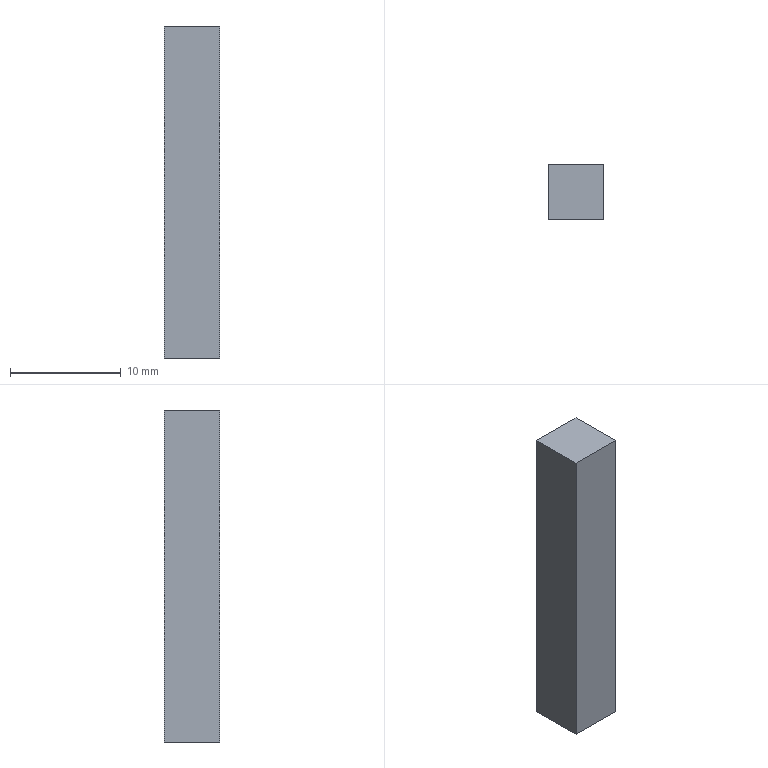Part | STEP file | BCC3 H16_16 | 1 solid | 6 faces | box 5 x 5 x 30 mm | volume 750 mm3 | plane 6
STEP:
#1=CARTESIAN_POINT('',(0.,0.,0.));
#2=DIRECTION('',(0.,0.,1.));
#3=DIRECTION('',(1.,0.,0.));
#4=AXIS2_PLACEMENT_3D('',#1,#2,#3);
#5=CARTESIAN_POINT('',(-2.5,2.5,-15.));
#6=VERTEX_POINT('',#5);
#7=CARTESIAN_POINT('',(-2.5,-2.5,-15.));
#8=VERTEX_POINT('',#7);
#9=CARTESIAN_POINT('',(-2.5,2.5,-15.));
#10=DIRECTION('',(0.,-1.,0.));
#11=VECTOR('',#10,1.);
#12=LINE('',#9,#11);
#13=CARTESIAN_POINT('',(-2.5,2.5,15.));
#14=DIRECTION('',(1.,0.,0.));
#15=DIRECTION('',(0.,0.,-1.));
#16=AXIS2_PLACEMENT_3D('',#13,#14,#15);
#17=PLANE('',#16);
#18=CARTESIAN_POINT('',(30.,0.));
#19=DIRECTION('',(0.,-1.));
#20=VECTOR('',#19,1.);
#21=LINE('',#18,#20);
#22=(GEOMETRIC_REPRESENTATION_CONTEXT(2)PARAMETRIC_REPRESENTATION_CONTEXT()REPRESENTATION_CONTEXT('',''));
#23=DEFINITIONAL_REPRESENTATION('',(#21),#22);
#24=PCURVE('',#17,#23);
#25=CARTESIAN_POINT('',(0.,0.,-15.));
#26=DIRECTION('',(0.,0.,1.));
#27=DIRECTION('',(1.,0.,0.));
#28=AXIS2_PLACEMENT_3D('',#25,#26,#27);
#29=PLANE('',#28);
#30=CARTESIAN_POINT('',(-2.5,2.5));
#31=DIRECTION('',(0.,-1.));
#32=VECTOR('',#31,1.);
#33=LINE('',#30,#32);
#34=(GEOMETRIC_REPRESENTATION_CONTEXT(2)PARAMETRIC_REPRESENTATION_CONTEXT()REPRESENTATION_CONTEXT('',''));
#35=DEFINITIONAL_REPRESENTATION('',(#33),#34);
#36=PCURVE('',#29,#35);
#37=SURFACE_CURVE('',#12,(#24,#36),.PCURVE_S1.);
#38=EDGE_CURVE('',#6,#8,#37,.T.);
#39=ORIENTED_EDGE('',*,*,#38,.T.);
#40=CARTESIAN_POINT('',(-2.5,-2.5,15.));
#41=VERTEX_POINT('',#40);
#42=CARTESIAN_POINT('',(-2.5,-2.5,15.));
#43=DIRECTION('',(0.,0.,-1.));
#44=VECTOR('',#43,1.);
#45=LINE('',#42,#44);
#46=CARTESIAN_POINT('',(0.,-5.));
#47=DIRECTION('',(1.,0.));
#48=VECTOR('',#47,1.);
#49=LINE('',#46,#48);
#50=(GEOMETRIC_REPRESENTATION_CONTEXT(2)PARAMETRIC_REPRESENTATION_CONTEXT()REPRESENTATION_CONTEXT('',''));
#51=DEFINITIONAL_REPRESENTATION('',(#49),#50);
#52=PCURVE('',#17,#51);
#53=CARTESIAN_POINT('',(-2.5,-2.5,15.));
#54=DIRECTION('',(0.,1.,0.));
#55=DIRECTION('',(-1.,0.,0.));
#56=AXIS2_PLACEMENT_3D('',#53,#54,#55);
#57=PLANE('',#56);
#58=CARTESIAN_POINT('',(0.,0.));
#59=DIRECTION('',(0.,-1.));
#60=VECTOR('',#59,1.);
#61=LINE('',#58,#60);
#62=(GEOMETRIC_REPRESENTATION_CONTEXT(2)PARAMETRIC_REPRESENTATION_CONTEXT()REPRESENTATION_CONTEXT('',''));
#63=DEFINITIONAL_REPRESENTATION('',(#61),#62);
#64=PCURVE('',#57,#63);
#65=SURFACE_CURVE('',#45,(#52,#64),.PCURVE_S1.);
#66=EDGE_CURVE('',#41,#8,#65,.T.);
#67=ORIENTED_EDGE('',*,*,#66,.F.);
#68=CARTESIAN_POINT('',(-2.5,2.5,15.));
#69=VERTEX_POINT('',#68);
#70=CARTESIAN_POINT('',(-2.5,2.5,15.));
#71=DIRECTION('',(0.,-1.,0.));
#72=VECTOR('',#71,1.);
#73=LINE('',#70,#72);
#74=CARTESIAN_POINT('',(0.,0.));
#75=DIRECTION('',(0.,-1.));
#76=VECTOR('',#75,1.);
#77=LINE('',#74,#76);
#78=(GEOMETRIC_REPRESENTATION_CONTEXT(2)PARAMETRIC_REPRESENTATION_CONTEXT()REPRESENTATION_CONTEXT('',''));
#79=DEFINITIONAL_REPRESENTATION('',(#77),#78);
#80=PCURVE('',#17,#79);
#81=CARTESIAN_POINT('',(0.,0.,15.));
#82=DIRECTION('',(0.,0.,1.));
#83=DIRECTION('',(1.,0.,0.));
#84=AXIS2_PLACEMENT_3D('',#81,#82,#83);
#85=PLANE('',#84);
#86=CARTESIAN_POINT('',(-2.5,2.5));
#87=DIRECTION('',(0.,-1.));
#88=VECTOR('',#87,1.);
#89=LINE('',#86,#88);
#90=(GEOMETRIC_REPRESENTATION_CONTEXT(2)PARAMETRIC_REPRESENTATION_CONTEXT()REPRESENTATION_CONTEXT('',''));
#91=DEFINITIONAL_REPRESENTATION('',(#89),#90);
#92=PCURVE('',#85,#91);
#93=SURFACE_CURVE('',#73,(#80,#92),.PCURVE_S1.);
#94=EDGE_CURVE('',#69,#41,#93,.T.);
#95=ORIENTED_EDGE('',*,*,#94,.F.);
#96=CARTESIAN_POINT('',(-2.5,2.5,15.));
#97=DIRECTION('',(0.,0.,-1.));
#98=VECTOR('',#97,1.);
#99=LINE('',#96,#98);
#100=CARTESIAN_POINT('',(0.,0.));
#101=DIRECTION('',(1.,0.));
#102=VECTOR('',#101,1.);
#103=LINE('',#100,#102);
#104=(GEOMETRIC_REPRESENTATION_CONTEXT(2)PARAMETRIC_REPRESENTATION_CONTEXT()REPRESENTATION_CONTEXT('',''));
#105=DEFINITIONAL_REPRESENTATION('',(#103),#104);
#106=PCURVE('',#17,#105);
#107=CARTESIAN_POINT('',(-2.5,2.5,15.));
#108=DIRECTION('',(0.,-1.,0.));
#109=DIRECTION('',(0.,0.,-1.));
#110=AXIS2_PLACEMENT_3D('',#107,#108,#109);
#111=PLANE('',#110);
#112=CARTESIAN_POINT('',(0.,0.));
#113=DIRECTION('',(1.,0.));
#114=VECTOR('',#113,1.);
#115=LINE('',#112,#114);
#116=(GEOMETRIC_REPRESENTATION_CONTEXT(2)PARAMETRIC_REPRESENTATION_CONTEXT()REPRESENTATION_CONTEXT('',''));
#117=DEFINITIONAL_REPRESENTATION('',(#115),#116);
#118=PCURVE('',#111,#117);
#119=SURFACE_CURVE('',#99,(#106,#118),.PCURVE_S1.);
#120=EDGE_CURVE('',#69,#6,#119,.T.);
#121=ORIENTED_EDGE('',*,*,#120,.T.);
#122=EDGE_LOOP('',(#39,#67,#95,#121));
#123=FACE_BOUND('',#122,.T.);
#124=ADVANCED_FACE('',(#123),#17,.F.);
#125=CARTESIAN_POINT('',(2.5,-2.5,-15.));
#126=VERTEX_POINT('',#125);
#127=CARTESIAN_POINT('',(-2.5,-2.5,-15.));
#128=DIRECTION('',(1.,0.,0.));
#129=VECTOR('',#128,1.);
#130=LINE('',#127,#129);
#131=CARTESIAN_POINT('',(0.,-30.));
#132=DIRECTION('',(-1.,0.));
#133=VECTOR('',#132,1.);
#134=LINE('',#131,#133);
#135=(GEOMETRIC_REPRESENTATION_CONTEXT(2)PARAMETRIC_REPRESENTATION_CONTEXT()REPRESENTATION_CONTEXT('',''));
#136=DEFINITIONAL_REPRESENTATION('',(#134),#135);
#137=PCURVE('',#57,#136);
#138=CARTESIAN_POINT('',(-2.5,-2.5));
#139=DIRECTION('',(1.,0.));
#140=VECTOR('',#139,1.);
#141=LINE('',#138,#140);
#142=(GEOMETRIC_REPRESENTATION_CONTEXT(2)PARAMETRIC_REPRESENTATION_CONTEXT()REPRESENTATION_CONTEXT('',''));
#143=DEFINITIONAL_REPRESENTATION('',(#141),#142);
#144=PCURVE('',#29,#143);
#145=SURFACE_CURVE('',#130,(#137,#144),.PCURVE_S1.);
#146=EDGE_CURVE('',#8,#126,#145,.T.);
#147=ORIENTED_EDGE('',*,*,#146,.T.);
#148=CARTESIAN_POINT('',(2.5,-2.5,15.));
#149=VERTEX_POINT('',#148);
#150=CARTESIAN_POINT('',(2.5,-2.5,15.));
#151=DIRECTION('',(0.,0.,-1.));
#152=VECTOR('',#151,1.);
#153=LINE('',#150,#152);
#154=CARTESIAN_POINT('',(-5.,0.));
#155=DIRECTION('',(0.,-1.));
#156=VECTOR('',#155,1.);
#157=LINE('',#154,#156);
#158=(GEOMETRIC_REPRESENTATION_CONTEXT(2)PARAMETRIC_REPRESENTATION_CONTEXT()REPRESENTATION_CONTEXT('',''));
#159=DEFINITIONAL_REPRESENTATION('',(#157),#158);
#160=PCURVE('',#57,#159);
#161=CARTESIAN_POINT('',(2.5,2.5,15.));
#162=DIRECTION('',(-1.,0.,0.));
#163=DIRECTION('',(0.,0.,1.));
#164=AXIS2_PLACEMENT_3D('',#161,#162,#163);
#165=PLANE('',#164);
#166=CARTESIAN_POINT('',(0.,-5.));
#167=DIRECTION('',(-1.,0.));
#168=VECTOR('',#167,1.);
#169=LINE('',#166,#168);
#170=(GEOMETRIC_REPRESENTATION_CONTEXT(2)PARAMETRIC_REPRESENTATION_CONTEXT()REPRESENTATION_CONTEXT('',''));
#171=DEFINITIONAL_REPRESENTATION('',(#169),#170);
#172=PCURVE('',#165,#171);
#173=SURFACE_CURVE('',#153,(#160,#172),.PCURVE_S1.);
#174=EDGE_CURVE('',#149,#126,#173,.T.);
#175=ORIENTED_EDGE('',*,*,#174,.F.);
#176=CARTESIAN_POINT('',(-2.5,-2.5,15.));
#177=DIRECTION('',(1.,0.,0.));
#178=VECTOR('',#177,1.);
#179=LINE('',#176,#178);
#180=CARTESIAN_POINT('',(0.,0.));
#181=DIRECTION('',(-1.,0.));
#182=VECTOR('',#181,1.);
#183=LINE('',#180,#182);
#184=(GEOMETRIC_REPRESENTATION_CONTEXT(2)PARAMETRIC_REPRESENTATION_CONTEXT()REPRESENTATION_CONTEXT('',''));
#185=DEFINITIONAL_REPRESENTATION('',(#183),#184);
#186=PCURVE('',#57,#185);
#187=CARTESIAN_POINT('',(-2.5,-2.5));
#188=DIRECTION('',(1.,0.));
#189=VECTOR('',#188,1.);
#190=LINE('',#187,#189);
#191=(GEOMETRIC_REPRESENTATION_CONTEXT(2)PARAMETRIC_REPRESENTATION_CONTEXT()REPRESENTATION_CONTEXT('',''));
#192=DEFINITIONAL_REPRESENTATION('',(#190),#191);
#193=PCURVE('',#85,#192);
#194=SURFACE_CURVE('',#179,(#186,#193),.PCURVE_S1.);
#195=EDGE_CURVE('',#41,#149,#194,.T.);
#196=ORIENTED_EDGE('',*,*,#195,.F.);
#197=ORIENTED_EDGE('',*,*,#66,.T.);
#198=EDGE_LOOP('',(#147,#175,#196,#197));
#199=FACE_BOUND('',#198,.T.);
#200=ADVANCED_FACE('',(#199),#57,.F.);
#201=CARTESIAN_POINT('',(2.5,2.5,-15.));
#202=VERTEX_POINT('',#201);
#203=CARTESIAN_POINT('',(2.5,2.5,-15.));
#204=DIRECTION('',(0.,1.,0.));
#205=VECTOR('',#204,1.);
#206=LINE('',#203,#205);
#207=CARTESIAN_POINT('',(-30.,0.));
#208=DIRECTION('',(0.,1.));
#209=VECTOR('',#208,1.);
#210=LINE('',#207,#209);
#211=(GEOMETRIC_REPRESENTATION_CONTEXT(2)PARAMETRIC_REPRESENTATION_CONTEXT()REPRESENTATION_CONTEXT('',''));
#212=DEFINITIONAL_REPRESENTATION('',(#210),#211);
#213=PCURVE('',#165,#212);
#214=CARTESIAN_POINT('',(2.5,2.5));
#215=DIRECTION('',(0.,1.));
#216=VECTOR('',#215,1.);
#217=LINE('',#214,#216);
#218=(GEOMETRIC_REPRESENTATION_CONTEXT(2)PARAMETRIC_REPRESENTATION_CONTEXT()REPRESENTATION_CONTEXT('',''));
#219=DEFINITIONAL_REPRESENTATION('',(#217),#218);
#220=PCURVE('',#29,#219);
#221=SURFACE_CURVE('',#206,(#213,#220),.PCURVE_S1.);
#222=EDGE_CURVE('',#126,#202,#221,.T.);
#223=ORIENTED_EDGE('',*,*,#222,.T.);
#224=CARTESIAN_POINT('',(2.5,2.5,15.));
#225=VERTEX_POINT('',#224);
#226=CARTESIAN_POINT('',(2.5,2.5,15.));
#227=DIRECTION('',(0.,0.,-1.));
#228=VECTOR('',#227,1.);
#229=LINE('',#226,#228);
#230=CARTESIAN_POINT('',(0.,0.));
#231=DIRECTION('',(-1.,0.));
#232=VECTOR('',#231,1.);
#233=LINE('',#230,#232);
#234=(GEOMETRIC_REPRESENTATION_CONTEXT(2)PARAMETRIC_REPRESENTATION_CONTEXT()REPRESENTATION_CONTEXT('',''));
#235=DEFINITIONAL_REPRESENTATION('',(#233),#234);
#236=PCURVE('',#165,#235);
#237=CARTESIAN_POINT('',(0.,5.));
#238=DIRECTION('',(1.,0.));
#239=VECTOR('',#238,1.);
#240=LINE('',#237,#239);
#241=(GEOMETRIC_REPRESENTATION_CONTEXT(2)PARAMETRIC_REPRESENTATION_CONTEXT()REPRESENTATION_CONTEXT('',''));
#242=DEFINITIONAL_REPRESENTATION('',(#240),#241);
#243=PCURVE('',#111,#242);
#244=SURFACE_CURVE('',#229,(#236,#243),.PCURVE_S1.);
#245=EDGE_CURVE('',#225,#202,#244,.T.);
#246=ORIENTED_EDGE('',*,*,#245,.F.);
#247=CARTESIAN_POINT('',(2.5,2.5,15.));
#248=DIRECTION('',(0.,1.,0.));
#249=VECTOR('',#248,1.);
#250=LINE('',#247,#249);
#251=CARTESIAN_POINT('',(0.,0.));
#252=DIRECTION('',(0.,1.));
#253=VECTOR('',#252,1.);
#254=LINE('',#251,#253);
#255=(GEOMETRIC_REPRESENTATION_CONTEXT(2)PARAMETRIC_REPRESENTATION_CONTEXT()REPRESENTATION_CONTEXT('',''));
#256=DEFINITIONAL_REPRESENTATION('',(#254),#255);
#257=PCURVE('',#165,#256);
#258=CARTESIAN_POINT('',(2.5,2.5));
#259=DIRECTION('',(0.,1.));
#260=VECTOR('',#259,1.);
#261=LINE('',#258,#260);
#262=(GEOMETRIC_REPRESENTATION_CONTEXT(2)PARAMETRIC_REPRESENTATION_CONTEXT()REPRESENTATION_CONTEXT('',''));
#263=DEFINITIONAL_REPRESENTATION('',(#261),#262);
#264=PCURVE('',#85,#263);
#265=SURFACE_CURVE('',#250,(#257,#264),.PCURVE_S1.);
#266=EDGE_CURVE('',#149,#225,#265,.T.);
#267=ORIENTED_EDGE('',*,*,#266,.F.);
#268=ORIENTED_EDGE('',*,*,#174,.T.);
#269=EDGE_LOOP('',(#223,#246,#267,#268));
#270=FACE_BOUND('',#269,.T.);
#271=ADVANCED_FACE('',(#270),#165,.F.);
#272=CARTESIAN_POINT('',(-2.5,2.5,-15.));
#273=DIRECTION('',(-1.,0.,0.));
#274=VECTOR('',#273,1.);
#275=LINE('',#272,#274);
#276=CARTESIAN_POINT('',(30.,0.));
#277=DIRECTION('',(0.,-1.));
#278=VECTOR('',#277,1.);
#279=LINE('',#276,#278);
#280=(GEOMETRIC_REPRESENTATION_CONTEXT(2)PARAMETRIC_REPRESENTATION_CONTEXT()REPRESENTATION_CONTEXT('',''));
#281=DEFINITIONAL_REPRESENTATION('',(#279),#280);
#282=PCURVE('',#111,#281);
#283=CARTESIAN_POINT('',(-2.5,2.5));
#284=DIRECTION('',(-1.,0.));
#285=VECTOR('',#284,1.);
#286=LINE('',#283,#285);
#287=(GEOMETRIC_REPRESENTATION_CONTEXT(2)PARAMETRIC_REPRESENTATION_CONTEXT()REPRESENTATION_CONTEXT('',''));
#288=DEFINITIONAL_REPRESENTATION('',(#286),#287);
#289=PCURVE('',#29,#288);
#290=SURFACE_CURVE('',#275,(#282,#289),.PCURVE_S1.);
#291=EDGE_CURVE('',#202,#6,#290,.T.);
#292=ORIENTED_EDGE('',*,*,#291,.T.);
#293=ORIENTED_EDGE('',*,*,#120,.F.);
#294=CARTESIAN_POINT('',(-2.5,2.5,15.));
#295=DIRECTION('',(-1.,0.,0.));
#296=VECTOR('',#295,1.);
#297=LINE('',#294,#296);
#298=CARTESIAN_POINT('',(0.,0.));
#299=DIRECTION('',(0.,-1.));
#300=VECTOR('',#299,1.);
#301=LINE('',#298,#300);
#302=(GEOMETRIC_REPRESENTATION_CONTEXT(2)PARAMETRIC_REPRESENTATION_CONTEXT()REPRESENTATION_CONTEXT('',''));
#303=DEFINITIONAL_REPRESENTATION('',(#301),#302);
#304=PCURVE('',#111,#303);
#305=CARTESIAN_POINT('',(-2.5,2.5));
#306=DIRECTION('',(-1.,0.));
#307=VECTOR('',#306,1.);
#308=LINE('',#305,#307);
#309=(GEOMETRIC_REPRESENTATION_CONTEXT(2)PARAMETRIC_REPRESENTATION_CONTEXT()REPRESENTATION_CONTEXT('',''));
#310=DEFINITIONAL_REPRESENTATION('',(#308),#309);
#311=PCURVE('',#85,#310);
#312=SURFACE_CURVE('',#297,(#304,#311),.PCURVE_S1.);
#313=EDGE_CURVE('',#225,#69,#312,.T.);
#314=ORIENTED_EDGE('',*,*,#313,.F.);
#315=ORIENTED_EDGE('',*,*,#245,.T.);
#316=EDGE_LOOP('',(#292,#293,#314,#315));
#317=FACE_BOUND('',#316,.T.);
#318=ADVANCED_FACE('',(#317),#111,.F.);
#319=ORIENTED_EDGE('',*,*,#94,.T.);
#320=ORIENTED_EDGE('',*,*,#195,.T.);
#321=ORIENTED_EDGE('',*,*,#266,.T.);
#322=ORIENTED_EDGE('',*,*,#313,.T.);
#323=EDGE_LOOP('',(#319,#320,#321,#322));
#324=FACE_BOUND('',#323,.T.);
#325=ADVANCED_FACE('',(#324),#85,.T.);
#326=ORIENTED_EDGE('',*,*,#38,.F.);
#327=ORIENTED_EDGE('',*,*,#291,.F.);
#328=ORIENTED_EDGE('',*,*,#222,.F.);
#329=ORIENTED_EDGE('',*,*,#146,.F.);
#330=EDGE_LOOP('',(#326,#327,#328,#329));
#331=FACE_BOUND('',#330,.T.);
#332=ADVANCED_FACE('',(#331),#29,.F.);
#333=CLOSED_SHELL('',(#124,#200,#271,#318,#325,#332));
#334=MANIFOLD_SOLID_BREP('',#333);
#335=(LENGTH_UNIT()NAMED_UNIT(*)SI_UNIT(.MILLI.,.METRE.));
#336=UNCERTAINTY_MEASURE_WITH_UNIT(LENGTH_MEASURE(0.0000001),#335,'','');
#337=(NAMED_UNIT(*)PLANE_ANGLE_UNIT()SI_UNIT($,.RADIAN.));
#338=(NAMED_UNIT(*)SI_UNIT($,.STERADIAN.)SOLID_ANGLE_UNIT());
#339=(GEOMETRIC_REPRESENTATION_CONTEXT(3)GLOBAL_UNCERTAINTY_ASSIGNED_CONTEXT((#336))GLOBAL_UNIT_ASSIGNED_CONTEXT((#335,#337,#338))REPRESENTATION_CONTEXT('',''));
#340=ADVANCED_BREP_SHAPE_REPRESENTATION('',(#4,#334),#339);